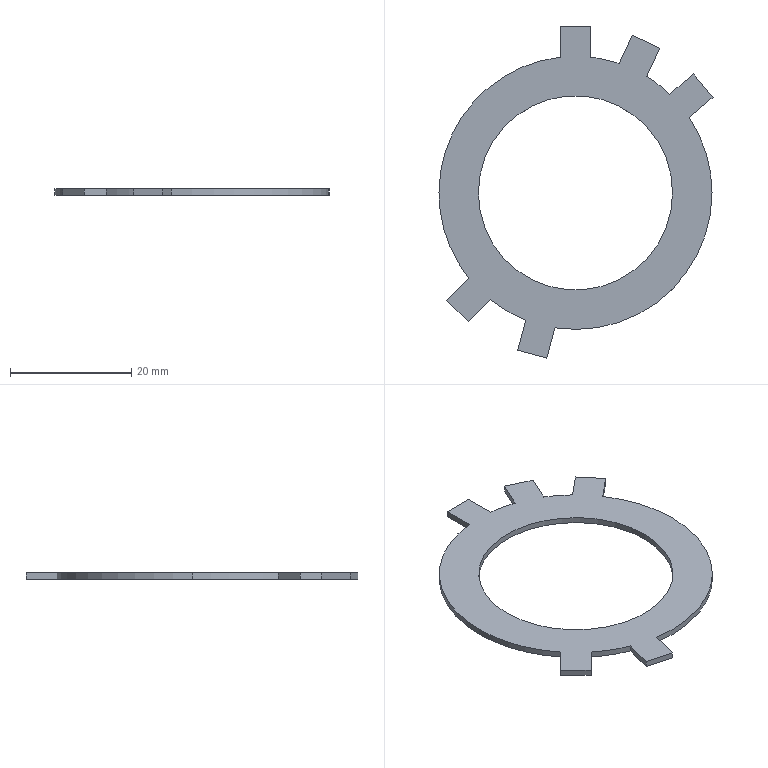Part | STEP file | ZDDQ | 1 solid | 26 faces | box 45.173 x 54.71 x 1 mm | volume 912.343 mm3 | plane 17 | cylinder 9 | commonest cylinder face diameters 45 x7 32 x2
STEP:
#1=CARTESIAN_POINT('',(-9.532,-25.916,0.));
#2=VERTEX_POINT('',#1);
#3=CARTESIAN_POINT('',(-4.703,-27.21,0.));
#4=VERTEX_POINT('',#3);
#5=CARTESIAN_POINT('',(-7.118,-26.563,0.));
#6=DIRECTION('',(-0.9659,0.2588,0.));
#7=VECTOR('',#6,1.);
#8=LINE('',#5,#7);
#9=EDGE_CURVE('',#2,#4,#8,.F.);
#10=ORIENTED_EDGE('',*,*,#9,.T.);
#11=CARTESIAN_POINT('',(-4.703,-27.21,1.));
#12=VERTEX_POINT('',#11);
#13=CARTESIAN_POINT('',(-4.703,-27.21,0.5));
#14=DIRECTION('',(0.,0.,-1.));
#15=VECTOR('',#14,1.);
#16=LINE('',#13,#15);
#17=EDGE_CURVE('',#12,#4,#16,.T.);
#18=ORIENTED_EDGE('',*,*,#17,.F.);
#19=CARTESIAN_POINT('',(-9.532,-25.916,1.));
#20=VERTEX_POINT('',#19);
#21=CARTESIAN_POINT('',(-7.118,-26.563,1.));
#22=DIRECTION('',(-0.9659,0.2588,0.));
#23=VECTOR('',#22,1.);
#24=LINE('',#21,#23);
#25=EDGE_CURVE('',#20,#12,#24,.F.);
#26=ORIENTED_EDGE('',*,*,#25,.F.);
#27=CARTESIAN_POINT('',(-9.532,-25.916,0.5));
#28=DIRECTION('',(0.,0.,-1.));
#29=VECTOR('',#28,1.);
#30=LINE('',#27,#29);
#31=EDGE_CURVE('',#20,#2,#30,.T.);
#32=ORIENTED_EDGE('',*,*,#31,.T.);
#33=EDGE_LOOP('',(#10,#18,#26,#32));
#34=FACE_OUTER_BOUND('',#33,.T.);
#35=CARTESIAN_POINT('',(-4.703,-27.21,1.));
#36=DIRECTION('',(-0.2588,-0.9659,0.));
#37=DIRECTION('',(-0.9659,0.2588,0.));
#38=AXIS2_PLACEMENT_3D('',#35,#36,#37);
#39=PLANE('',#38);
#40=ADVANCED_FACE('',(#34),#39,.T.);
#41=CARTESIAN_POINT('',(-3.373,-22.246,0.));
#42=VERTEX_POINT('',#41);
#43=CARTESIAN_POINT('',(-3.373,-22.246,1.));
#44=VERTEX_POINT('',#43);
#45=CARTESIAN_POINT('',(-3.373,-22.246,0.5));
#46=DIRECTION('',(0.,0.,1.));
#47=VECTOR('',#46,1.);
#48=LINE('',#45,#47);
#49=EDGE_CURVE('',#42,#44,#48,.T.);
#50=ORIENTED_EDGE('',*,*,#49,.T.);
#51=CARTESIAN_POINT('',(-4.038,-24.728,1.));
#52=DIRECTION('',(0.2588,0.9659,0.));
#53=VECTOR('',#52,1.);
#54=LINE('',#51,#53);
#55=EDGE_CURVE('',#12,#44,#54,.T.);
#56=ORIENTED_EDGE('',*,*,#55,.F.);
#57=ORIENTED_EDGE('',*,*,#17,.T.);
#58=CARTESIAN_POINT('',(-4.038,-24.728,0.));
#59=DIRECTION('',(0.2588,0.9659,0.));
#60=VECTOR('',#59,1.);
#61=LINE('',#58,#60);
#62=EDGE_CURVE('',#4,#42,#61,.T.);
#63=ORIENTED_EDGE('',*,*,#62,.T.);
#64=EDGE_LOOP('',(#50,#56,#57,#63));
#65=FACE_OUTER_BOUND('',#64,.T.);
#66=CARTESIAN_POINT('',(-4.703,-27.21,1.));
#67=DIRECTION('',(-0.9659,0.2588,0.));
#68=DIRECTION('',(0.2588,0.9659,0.));
#69=AXIS2_PLACEMENT_3D('',#66,#67,#68);
#70=PLANE('',#69);
#71=ADVANCED_FACE('',(#65),#70,.F.);
#72=CARTESIAN_POINT('',(-8.202,-20.952,0.));
#73=VERTEX_POINT('',#72);
#74=CARTESIAN_POINT('',(-8.202,-20.952,1.));
#75=VERTEX_POINT('',#74);
#76=CARTESIAN_POINT('',(-8.202,-20.952,0.5));
#77=DIRECTION('',(0.,0.,1.));
#78=VECTOR('',#77,1.);
#79=LINE('',#76,#78);
#80=EDGE_CURVE('',#73,#75,#79,.T.);
#81=ORIENTED_EDGE('',*,*,#80,.F.);
#82=CARTESIAN_POINT('',(-8.867,-23.434,0.));
#83=DIRECTION('',(-0.2588,-0.9659,0.));
#84=VECTOR('',#83,1.);
#85=LINE('',#82,#84);
#86=EDGE_CURVE('',#73,#2,#85,.T.);
#87=ORIENTED_EDGE('',*,*,#86,.T.);
#88=ORIENTED_EDGE('',*,*,#31,.F.);
#89=CARTESIAN_POINT('',(-8.867,-23.434,1.));
#90=DIRECTION('',(-0.2588,-0.9659,0.));
#91=VECTOR('',#90,1.);
#92=LINE('',#89,#91);
#93=EDGE_CURVE('',#75,#20,#92,.T.);
#94=ORIENTED_EDGE('',*,*,#93,.F.);
#95=EDGE_LOOP('',(#81,#87,#88,#94));
#96=FACE_OUTER_BOUND('',#95,.T.);
#97=CARTESIAN_POINT('',(-6.944,-16.257,1.));
#98=DIRECTION('',(0.9659,-0.2588,0.));
#99=DIRECTION('',(-0.2588,-0.9659,0.));
#100=AXIS2_PLACEMENT_3D('',#97,#98,#99);
#101=PLANE('',#100);
#102=ADVANCED_FACE('',(#96),#101,.F.);
#103=CARTESIAN_POINT('',(-21.213,-17.678,0.));
#104=VERTEX_POINT('',#103);
#105=CARTESIAN_POINT('',(-17.678,-21.213,0.));
#106=VERTEX_POINT('',#105);
#107=CARTESIAN_POINT('',(-19.445,-19.445,0.));
#108=DIRECTION('',(-0.7071,0.7071,0.));
#109=VECTOR('',#108,1.);
#110=LINE('',#107,#109);
#111=EDGE_CURVE('',#104,#106,#110,.F.);
#112=ORIENTED_EDGE('',*,*,#111,.T.);
#113=CARTESIAN_POINT('',(-17.678,-21.213,1.));
#114=VERTEX_POINT('',#113);
#115=CARTESIAN_POINT('',(-17.678,-21.213,0.5));
#116=DIRECTION('',(0.,0.,-1.));
#117=VECTOR('',#116,1.);
#118=LINE('',#115,#117);
#119=EDGE_CURVE('',#114,#106,#118,.T.);
#120=ORIENTED_EDGE('',*,*,#119,.F.);
#121=CARTESIAN_POINT('',(-21.213,-17.678,1.));
#122=VERTEX_POINT('',#121);
#123=CARTESIAN_POINT('',(-19.445,-19.445,1.));
#124=DIRECTION('',(-0.7071,0.7071,0.));
#125=VECTOR('',#124,1.);
#126=LINE('',#123,#125);
#127=EDGE_CURVE('',#122,#114,#126,.F.);
#128=ORIENTED_EDGE('',*,*,#127,.F.);
#129=CARTESIAN_POINT('',(-21.213,-17.678,0.5));
#130=DIRECTION('',(0.,0.,-1.));
#131=VECTOR('',#130,1.);
#132=LINE('',#129,#131);
#133=EDGE_CURVE('',#122,#104,#132,.T.);
#134=ORIENTED_EDGE('',*,*,#133,.T.);
#135=EDGE_LOOP('',(#112,#120,#128,#134));
#136=FACE_OUTER_BOUND('',#135,.T.);
#137=CARTESIAN_POINT('',(-17.678,-21.213,1.));
#138=DIRECTION('',(-0.7071,-0.7071,0.));
#139=DIRECTION('',(-0.7071,0.7071,0.));
#140=AXIS2_PLACEMENT_3D('',#137,#138,#139);
#141=PLANE('',#140);
#142=ADVANCED_FACE('',(#136),#141,.T.);
#143=CARTESIAN_POINT('',(-14.044,-17.579,0.));
#144=VERTEX_POINT('',#143);
#145=CARTESIAN_POINT('',(-14.044,-17.579,1.));
#146=VERTEX_POINT('',#145);
#147=CARTESIAN_POINT('',(-14.044,-17.579,0.5));
#148=DIRECTION('',(0.,0.,1.));
#149=VECTOR('',#148,1.);
#150=LINE('',#147,#149);
#151=EDGE_CURVE('',#144,#146,#150,.T.);
#152=ORIENTED_EDGE('',*,*,#151,.T.);
#153=CARTESIAN_POINT('',(-15.861,-19.396,1.));
#154=DIRECTION('',(0.7071,0.7071,0.));
#155=VECTOR('',#154,1.);
#156=LINE('',#153,#155);
#157=EDGE_CURVE('',#114,#146,#156,.T.);
#158=ORIENTED_EDGE('',*,*,#157,.F.);
#159=ORIENTED_EDGE('',*,*,#119,.T.);
#160=CARTESIAN_POINT('',(-15.861,-19.396,0.));
#161=DIRECTION('',(0.7071,0.7071,0.));
#162=VECTOR('',#161,1.);
#163=LINE('',#160,#162);
#164=EDGE_CURVE('',#106,#144,#163,.T.);
#165=ORIENTED_EDGE('',*,*,#164,.T.);
#166=EDGE_LOOP('',(#152,#158,#159,#165));
#167=FACE_OUTER_BOUND('',#166,.T.);
#168=CARTESIAN_POINT('',(-17.678,-21.213,1.));
#169=DIRECTION('',(-0.7071,0.7071,0.));
#170=DIRECTION('',(0.7071,0.7071,0.));
#171=AXIS2_PLACEMENT_3D('',#168,#169,#170);
#172=PLANE('',#171);
#173=ADVANCED_FACE('',(#167),#172,.F.);
#174=CARTESIAN_POINT('',(-17.579,-14.044,0.));
#175=VERTEX_POINT('',#174);
#176=CARTESIAN_POINT('',(-17.579,-14.044,1.));
#177=VERTEX_POINT('',#176);
#178=CARTESIAN_POINT('',(-17.579,-14.044,0.5));
#179=DIRECTION('',(0.,0.,1.));
#180=VECTOR('',#179,1.);
#181=LINE('',#178,#180);
#182=EDGE_CURVE('',#175,#177,#181,.T.);
#183=ORIENTED_EDGE('',*,*,#182,.F.);
#184=CARTESIAN_POINT('',(-19.396,-15.861,0.));
#185=DIRECTION('',(-0.7071,-0.7071,0.));
#186=VECTOR('',#185,1.);
#187=LINE('',#184,#186);
#188=EDGE_CURVE('',#175,#104,#187,.T.);
#189=ORIENTED_EDGE('',*,*,#188,.T.);
#190=ORIENTED_EDGE('',*,*,#133,.F.);
#191=CARTESIAN_POINT('',(-19.396,-15.861,1.));
#192=DIRECTION('',(-0.7071,-0.7071,0.));
#193=VECTOR('',#192,1.);
#194=LINE('',#191,#193);
#195=EDGE_CURVE('',#177,#122,#194,.T.);
#196=ORIENTED_EDGE('',*,*,#195,.F.);
#197=EDGE_LOOP('',(#183,#189,#190,#196));
#198=FACE_OUTER_BOUND('',#197,.T.);
#199=CARTESIAN_POINT('',(-14.142,-10.607,1.));
#200=DIRECTION('',(0.7071,-0.7071,0.));
#201=DIRECTION('',(-0.7071,-0.7071,0.));
#202=AXIS2_PLACEMENT_3D('',#199,#200,#201);
#203=PLANE('',#202);
#204=ADVANCED_FACE('',(#198),#203,.F.);
#205=CARTESIAN_POINT('',(13.888,23.867,0.));
#206=VERTEX_POINT('',#205);
#207=CARTESIAN_POINT('',(9.356,25.98,0.));
#208=VERTEX_POINT('',#207);
#209=CARTESIAN_POINT('',(11.622,24.923,0.));
#210=DIRECTION('',(0.9063,-0.4226,0.));
#211=VECTOR('',#210,1.);
#212=LINE('',#209,#211);
#213=EDGE_CURVE('',#206,#208,#212,.F.);
#214=ORIENTED_EDGE('',*,*,#213,.T.);
#215=CARTESIAN_POINT('',(9.356,25.98,1.));
#216=VERTEX_POINT('',#215);
#217=CARTESIAN_POINT('',(9.356,25.98,0.5));
#218=DIRECTION('',(0.,0.,-1.));
#219=VECTOR('',#218,1.);
#220=LINE('',#217,#219);
#221=EDGE_CURVE('',#216,#208,#220,.T.);
#222=ORIENTED_EDGE('',*,*,#221,.F.);
#223=CARTESIAN_POINT('',(13.888,23.867,1.));
#224=VERTEX_POINT('',#223);
#225=CARTESIAN_POINT('',(11.622,24.923,1.));
#226=DIRECTION('',(0.9063,-0.4226,0.));
#227=VECTOR('',#226,1.);
#228=LINE('',#225,#227);
#229=EDGE_CURVE('',#224,#216,#228,.F.);
#230=ORIENTED_EDGE('',*,*,#229,.F.);
#231=CARTESIAN_POINT('',(13.888,23.867,0.5));
#232=DIRECTION('',(0.,0.,-1.));
#233=VECTOR('',#232,1.);
#234=LINE('',#231,#233);
#235=EDGE_CURVE('',#224,#206,#234,.T.);
#236=ORIENTED_EDGE('',*,*,#235,.T.);
#237=EDGE_LOOP('',(#214,#222,#230,#236));
#238=FACE_OUTER_BOUND('',#237,.T.);
#239=CARTESIAN_POINT('',(9.356,25.98,1.));
#240=DIRECTION('',(0.4226,0.9063,0.));
#241=DIRECTION('',(0.9063,-0.4226,0.));
#242=AXIS2_PLACEMENT_3D('',#239,#240,#241);
#243=PLANE('',#242);
#244=ADVANCED_FACE('',(#238),#243,.T.);
#245=CARTESIAN_POINT('',(7.184,21.322,0.));
#246=VERTEX_POINT('',#245);
#247=CARTESIAN_POINT('',(7.184,21.322,1.));
#248=VERTEX_POINT('',#247);
#249=CARTESIAN_POINT('',(7.184,21.322,0.5));
#250=DIRECTION('',(0.,0.,1.));
#251=VECTOR('',#250,1.);
#252=LINE('',#249,#251);
#253=EDGE_CURVE('',#246,#248,#252,.T.);
#254=ORIENTED_EDGE('',*,*,#253,.T.);
#255=CARTESIAN_POINT('',(8.27,23.651,1.));
#256=DIRECTION('',(-0.4226,-0.9063,0.));
#257=VECTOR('',#256,1.);
#258=LINE('',#255,#257);
#259=EDGE_CURVE('',#216,#248,#258,.T.);
#260=ORIENTED_EDGE('',*,*,#259,.F.);
#261=ORIENTED_EDGE('',*,*,#221,.T.);
#262=CARTESIAN_POINT('',(8.27,23.651,0.));
#263=DIRECTION('',(-0.4226,-0.9063,0.));
#264=VECTOR('',#263,1.);
#265=LINE('',#262,#264);
#266=EDGE_CURVE('',#208,#246,#265,.T.);
#267=ORIENTED_EDGE('',*,*,#266,.T.);
#268=EDGE_LOOP('',(#254,#260,#261,#267));
#269=FACE_OUTER_BOUND('',#268,.T.);
#270=CARTESIAN_POINT('',(9.356,25.98,1.));
#271=DIRECTION('',(0.9063,-0.4226,0.));
#272=DIRECTION('',(-0.4226,-0.9063,0.));
#273=AXIS2_PLACEMENT_3D('',#270,#271,#272);
#274=PLANE('',#273);
#275=ADVANCED_FACE('',(#269),#274,.F.);
#276=CARTESIAN_POINT('',(11.716,19.209,0.));
#277=VERTEX_POINT('',#276);
#278=CARTESIAN_POINT('',(11.716,19.209,1.));
#279=VERTEX_POINT('',#278);
#280=CARTESIAN_POINT('',(11.716,19.209,0.5));
#281=DIRECTION('',(0.,0.,1.));
#282=VECTOR('',#281,1.);
#283=LINE('',#280,#282);
#284=EDGE_CURVE('',#277,#279,#283,.T.);
#285=ORIENTED_EDGE('',*,*,#284,.F.);
#286=CARTESIAN_POINT('',(12.802,21.538,0.));
#287=DIRECTION('',(0.4226,0.9063,0.));
#288=VECTOR('',#287,1.);
#289=LINE('',#286,#288);
#290=EDGE_CURVE('',#277,#206,#289,.T.);
#291=ORIENTED_EDGE('',*,*,#290,.T.);
#292=ORIENTED_EDGE('',*,*,#235,.F.);
#293=CARTESIAN_POINT('',(12.802,21.538,1.));
#294=DIRECTION('',(0.4226,0.9063,0.));
#295=VECTOR('',#294,1.);
#296=LINE('',#293,#295);
#297=EDGE_CURVE('',#279,#224,#296,.T.);
#298=ORIENTED_EDGE('',*,*,#297,.F.);
#299=EDGE_LOOP('',(#285,#291,#292,#298));
#300=FACE_OUTER_BOUND('',#299,.T.);
#301=CARTESIAN_POINT('',(9.662,14.804,1.));
#302=DIRECTION('',(-0.9063,0.4226,0.));
#303=DIRECTION('',(0.4226,0.9063,0.));
#304=AXIS2_PLACEMENT_3D('',#301,#302,#303);
#305=PLANE('',#304);
#306=ADVANCED_FACE('',(#300),#305,.F.);
#307=CARTESIAN_POINT('',(22.673,15.762,0.));
#308=VERTEX_POINT('',#307);
#309=CARTESIAN_POINT('',(19.459,19.592,0.));
#310=VERTEX_POINT('',#309);
#311=CARTESIAN_POINT('',(21.066,17.677,0.));
#312=DIRECTION('',(0.6428,-0.766,0.));
#313=VECTOR('',#312,1.);
#314=LINE('',#311,#313);
#315=EDGE_CURVE('',#308,#310,#314,.F.);
#316=ORIENTED_EDGE('',*,*,#315,.T.);
#317=CARTESIAN_POINT('',(19.459,19.592,1.));
#318=VERTEX_POINT('',#317);
#319=CARTESIAN_POINT('',(19.459,19.592,0.5));
#320=DIRECTION('',(0.,0.,-1.));
#321=VECTOR('',#320,1.);
#322=LINE('',#319,#321);
#323=EDGE_CURVE('',#318,#310,#322,.T.);
#324=ORIENTED_EDGE('',*,*,#323,.F.);
#325=CARTESIAN_POINT('',(22.673,15.762,1.));
#326=VERTEX_POINT('',#325);
#327=CARTESIAN_POINT('',(21.066,17.677,1.));
#328=DIRECTION('',(0.6428,-0.766,0.));
#329=VECTOR('',#328,1.);
#330=LINE('',#327,#329);
#331=EDGE_CURVE('',#326,#318,#330,.F.);
#332=ORIENTED_EDGE('',*,*,#331,.F.);
#333=CARTESIAN_POINT('',(22.673,15.762,0.5));
#334=DIRECTION('',(0.,0.,-1.));
#335=VECTOR('',#334,1.);
#336=LINE('',#333,#335);
#337=EDGE_CURVE('',#326,#308,#336,.T.);
#338=ORIENTED_EDGE('',*,*,#337,.T.);
#339=EDGE_LOOP('',(#316,#324,#332,#338));
#340=FACE_OUTER_BOUND('',#339,.T.);
#341=CARTESIAN_POINT('',(19.459,19.592,1.));
#342=DIRECTION('',(0.766,0.6428,0.));
#343=DIRECTION('',(0.6428,-0.766,0.));
#344=AXIS2_PLACEMENT_3D('',#341,#342,#343);
#345=PLANE('',#344);
#346=ADVANCED_FACE('',(#340),#345,.T.);
#347=CARTESIAN_POINT('',(15.522,16.288,0.));
#348=VERTEX_POINT('',#347);
#349=CARTESIAN_POINT('',(15.522,16.288,1.));
#350=VERTEX_POINT('',#349);
#351=CARTESIAN_POINT('',(15.522,16.288,0.5));
#352=DIRECTION('',(0.,0.,1.));
#353=VECTOR('',#352,1.);
#354=LINE('',#351,#353);
#355=EDGE_CURVE('',#348,#350,#354,.T.);
#356=ORIENTED_EDGE('',*,*,#355,.T.);
#357=CARTESIAN_POINT('',(17.491,17.94,1.));
#358=DIRECTION('',(-0.766,-0.6428,0.));
#359=VECTOR('',#358,1.);
#360=LINE('',#357,#359);
#361=EDGE_CURVE('',#318,#350,#360,.T.);
#362=ORIENTED_EDGE('',*,*,#361,.F.);
#363=ORIENTED_EDGE('',*,*,#323,.T.);
#364=CARTESIAN_POINT('',(17.491,17.94,0.));
#365=DIRECTION('',(-0.766,-0.6428,0.));
#366=VECTOR('',#365,1.);
#367=LINE('',#364,#366);
#368=EDGE_CURVE('',#310,#348,#367,.T.);
#369=ORIENTED_EDGE('',*,*,#368,.T.);
#370=EDGE_LOOP('',(#356,#362,#363,#369));
#371=FACE_OUTER_BOUND('',#370,.T.);
#372=CARTESIAN_POINT('',(19.459,19.592,1.));
#373=DIRECTION('',(0.6428,-0.766,0.));
#374=DIRECTION('',(-0.766,-0.6428,0.));
#375=AXIS2_PLACEMENT_3D('',#372,#373,#374);
#376=PLANE('',#375);
#377=ADVANCED_FACE('',(#371),#376,.F.);
#378=CARTESIAN_POINT('',(18.736,12.458,0.));
#379=VERTEX_POINT('',#378);
#380=CARTESIAN_POINT('',(18.736,12.458,1.));
#381=VERTEX_POINT('',#380);
#382=CARTESIAN_POINT('',(18.736,12.458,0.5));
#383=DIRECTION('',(0.,0.,1.));
#384=VECTOR('',#383,1.);
#385=LINE('',#382,#384);
#386=EDGE_CURVE('',#379,#381,#385,.T.);
#387=ORIENTED_EDGE('',*,*,#386,.F.);
#388=CARTESIAN_POINT('',(20.705,14.11,0.));
#389=DIRECTION('',(0.766,0.6428,0.));
#390=VECTOR('',#389,1.);
#391=LINE('',#388,#390);
#392=EDGE_CURVE('',#379,#308,#391,.T.);
#393=ORIENTED_EDGE('',*,*,#392,.T.);
#394=ORIENTED_EDGE('',*,*,#337,.F.);
#395=CARTESIAN_POINT('',(20.705,14.11,1.));
#396=DIRECTION('',(0.766,0.6428,0.));
#397=VECTOR('',#396,1.);
#398=LINE('',#395,#397);
#399=EDGE_CURVE('',#381,#326,#398,.T.);
#400=ORIENTED_EDGE('',*,*,#399,.F.);
#401=EDGE_LOOP('',(#387,#393,#394,#400));
#402=FACE_OUTER_BOUND('',#401,.T.);
#403=CARTESIAN_POINT('',(15.013,9.334,1.));
#404=DIRECTION('',(-0.6428,0.766,0.));
#405=DIRECTION('',(0.766,0.6428,0.));
#406=AXIS2_PLACEMENT_3D('',#403,#404,#405);
#407=PLANE('',#406);
#408=ADVANCED_FACE('',(#402),#407,.F.);
#409=CARTESIAN_POINT('',(-16.,0.,1.));
#410=VERTEX_POINT('',#409);
#411=CARTESIAN_POINT('',(16.,0.,1.));
#412=VERTEX_POINT('',#411);
#413=CARTESIAN_POINT('',(0.,0.,1.));
#414=DIRECTION('',(0.,0.,1.));
#415=AXIS2_PLACEMENT_3D('',#413,#414,$);
#416=CIRCLE('',#415,16.);
#417=EDGE_CURVE('',#410,#412,#416,.T.);
#418=ORIENTED_EDGE('',*,*,#417,.T.);
#419=CARTESIAN_POINT('',(16.,0.,0.));
#420=VERTEX_POINT('',#419);
#421=CARTESIAN_POINT('',(16.,0.,0.5));
#422=DIRECTION('',(0.,0.,1.));
#423=VECTOR('',#422,1.);
#424=LINE('',#421,#423);
#425=EDGE_CURVE('',#420,#412,#424,.T.);
#426=ORIENTED_EDGE('',*,*,#425,.F.);
#427=CARTESIAN_POINT('',(-16.,0.,0.));
#428=VERTEX_POINT('',#427);
#429=CARTESIAN_POINT('',(0.,0.,0.));
#430=DIRECTION('',(0.,0.,1.));
#431=AXIS2_PLACEMENT_3D('',#429,#430,$);
#432=CIRCLE('',#431,16.);
#433=EDGE_CURVE('',#428,#420,#432,.T.);
#434=ORIENTED_EDGE('',*,*,#433,.F.);
#435=CARTESIAN_POINT('',(-16.,0.,0.5));
#436=DIRECTION('',(0.,0.,1.));
#437=VECTOR('',#436,1.);
#438=LINE('',#435,#437);
#439=EDGE_CURVE('',#428,#410,#438,.T.);
#440=ORIENTED_EDGE('',*,*,#439,.T.);
#441=EDGE_LOOP('',(#418,#426,#434,#440));
#442=FACE_OUTER_BOUND('',#441,.T.);
#443=CARTESIAN_POINT('',(0.,0.,0.5));
#444=DIRECTION('',(0.,0.,1.));
#445=DIRECTION('',(1.,0.,0.));
#446=AXIS2_PLACEMENT_3D('',#443,#444,#445);
#447=CYLINDRICAL_SURFACE('',#446,16.);
#448=ADVANCED_FACE('',(#442),#447,.F.);
#449=CARTESIAN_POINT('',(0.,0.,1.));
#450=DIRECTION('',(0.,0.,1.));
#451=AXIS2_PLACEMENT_3D('',#449,#450,$);
#452=CIRCLE('',#451,16.);
#453=EDGE_CURVE('',#412,#410,#452,.T.);
#454=ORIENTED_EDGE('',*,*,#453,.T.);
#455=ORIENTED_EDGE('',*,*,#439,.F.);
#456=CARTESIAN_POINT('',(0.,0.,0.));
#457=DIRECTION('',(0.,0.,1.));
#458=AXIS2_PLACEMENT_3D('',#456,#457,$);
#459=CIRCLE('',#458,16.);
#460=EDGE_CURVE('',#420,#428,#459,.T.);
#461=ORIENTED_EDGE('',*,*,#460,.F.);
#462=ORIENTED_EDGE('',*,*,#425,.T.);
#463=EDGE_LOOP('',(#454,#455,#461,#462));
#464=FACE_OUTER_BOUND('',#463,.T.);
#465=ADVANCED_FACE('',(#464),#447,.F.);
#466=CARTESIAN_POINT('',(0.,0.,0.));
#467=DIRECTION('',(0.,0.,1.));
#468=AXIS2_PLACEMENT_3D('',#466,#467,$);
#469=CIRCLE('',#468,22.5);
#470=EDGE_CURVE('',#348,#277,#469,.T.);
#471=ORIENTED_EDGE('',*,*,#470,.T.);
#472=ORIENTED_EDGE('',*,*,#284,.T.);
#473=CARTESIAN_POINT('',(0.,0.,1.));
#474=DIRECTION('',(0.,0.,1.));
#475=AXIS2_PLACEMENT_3D('',#473,#474,$);
#476=CIRCLE('',#475,22.5);
#477=EDGE_CURVE('',#350,#279,#476,.T.);
#478=ORIENTED_EDGE('',*,*,#477,.F.);
#479=ORIENTED_EDGE('',*,*,#355,.F.);
#480=EDGE_LOOP('',(#471,#472,#478,#479));
#481=FACE_OUTER_BOUND('',#480,.T.);
#482=CARTESIAN_POINT('',(0.,0.,0.5));
#483=DIRECTION('',(0.,0.,1.));
#484=DIRECTION('',(1.,0.,0.));
#485=AXIS2_PLACEMENT_3D('',#482,#483,#484);
#486=CYLINDRICAL_SURFACE('',#485,22.5);
#487=ADVANCED_FACE('',(#481),#486,.T.);
#488=ORIENTED_EDGE('',*,*,#253,.F.);
#489=CARTESIAN_POINT('',(2.5,22.361,0.));
#490=VERTEX_POINT('',#489);
#491=CARTESIAN_POINT('',(0.,0.,0.));
#492=DIRECTION('',(0.,0.,1.));
#493=AXIS2_PLACEMENT_3D('',#491,#492,$);
#494=CIRCLE('',#493,22.5);
#495=EDGE_CURVE('',#246,#490,#494,.T.);
#496=ORIENTED_EDGE('',*,*,#495,.T.);
#497=CARTESIAN_POINT('',(2.5,22.361,1.));
#498=VERTEX_POINT('',#497);
#499=CARTESIAN_POINT('',(2.5,22.361,0.5));
#500=DIRECTION('',(0.,0.,1.));
#501=VECTOR('',#500,1.);
#502=LINE('',#499,#501);
#503=EDGE_CURVE('',#490,#498,#502,.T.);
#504=ORIENTED_EDGE('',*,*,#503,.T.);
#505=CARTESIAN_POINT('',(0.,0.,1.));
#506=DIRECTION('',(0.,0.,1.));
#507=AXIS2_PLACEMENT_3D('',#505,#506,$);
#508=CIRCLE('',#507,22.5);
#509=EDGE_CURVE('',#248,#498,#508,.T.);
#510=ORIENTED_EDGE('',*,*,#509,.F.);
#511=EDGE_LOOP('',(#488,#496,#504,#510));
#512=FACE_OUTER_BOUND('',#511,.T.);
#513=ADVANCED_FACE('',(#512),#486,.T.);
#514=CARTESIAN_POINT('',(-2.5,22.361,0.));
#515=VERTEX_POINT('',#514);
#516=CARTESIAN_POINT('',(-22.5,0.,0.));
#517=VERTEX_POINT('',#516);
#518=CARTESIAN_POINT('',(0.,0.,0.));
#519=DIRECTION('',(0.,0.,1.));
#520=AXIS2_PLACEMENT_3D('',#518,#519,$);
#521=CIRCLE('',#520,22.5);
#522=EDGE_CURVE('',#515,#517,#521,.T.);
#523=ORIENTED_EDGE('',*,*,#522,.T.);
#524=CARTESIAN_POINT('',(-22.5,0.,1.));
#525=VERTEX_POINT('',#524);
#526=CARTESIAN_POINT('',(-22.5,0.,0.5));
#527=DIRECTION('',(0.,0.,1.));
#528=VECTOR('',#527,1.);
#529=LINE('',#526,#528);
#530=EDGE_CURVE('',#517,#525,#529,.T.);
#531=ORIENTED_EDGE('',*,*,#530,.T.);
#532=CARTESIAN_POINT('',(-2.5,22.361,1.));
#533=VERTEX_POINT('',#532);
#534=CARTESIAN_POINT('',(0.,0.,1.));
#535=DIRECTION('',(0.,0.,1.));
#536=AXIS2_PLACEMENT_3D('',#534,#535,$);
#537=CIRCLE('',#536,22.5);
#538=EDGE_CURVE('',#533,#525,#537,.T.);
#539=ORIENTED_EDGE('',*,*,#538,.F.);
#540=CARTESIAN_POINT('',(-2.5,22.361,0.5));
#541=DIRECTION('',(0.,0.,1.));
#542=VECTOR('',#541,1.);
#543=LINE('',#540,#542);
#544=EDGE_CURVE('',#515,#533,#543,.T.);
#545=ORIENTED_EDGE('',*,*,#544,.F.);
#546=EDGE_LOOP('',(#523,#531,#539,#545));
#547=FACE_OUTER_BOUND('',#546,.T.);
#548=ADVANCED_FACE('',(#547),#486,.T.);
#549=CARTESIAN_POINT('',(0.,0.,1.));
#550=DIRECTION('',(0.,0.,1.));
#551=AXIS2_PLACEMENT_3D('',#549,#550,$);
#552=CIRCLE('',#551,22.5);
#553=EDGE_CURVE('',#525,#177,#552,.T.);
#554=ORIENTED_EDGE('',*,*,#553,.F.);
#555=ORIENTED_EDGE('',*,*,#530,.F.);
#556=CARTESIAN_POINT('',(0.,0.,0.));
#557=DIRECTION('',(0.,0.,1.));
#558=AXIS2_PLACEMENT_3D('',#556,#557,$);
#559=CIRCLE('',#558,22.5);
#560=EDGE_CURVE('',#517,#175,#559,.T.);
#561=ORIENTED_EDGE('',*,*,#560,.T.);
#562=ORIENTED_EDGE('',*,*,#182,.T.);
#563=EDGE_LOOP('',(#554,#555,#561,#562));
#564=FACE_OUTER_BOUND('',#563,.T.);
#565=ADVANCED_FACE('',(#564),#486,.T.);
#566=CARTESIAN_POINT('',(0.,0.,0.));
#567=DIRECTION('',(0.,0.,1.));
#568=AXIS2_PLACEMENT_3D('',#566,#567,$);
#569=CIRCLE('',#568,22.5);
#570=EDGE_CURVE('',#144,#73,#569,.T.);
#571=ORIENTED_EDGE('',*,*,#570,.T.);
#572=ORIENTED_EDGE('',*,*,#80,.T.);
#573=CARTESIAN_POINT('',(0.,0.,1.));
#574=DIRECTION('',(0.,0.,1.));
#575=AXIS2_PLACEMENT_3D('',#573,#574,$);
#576=CIRCLE('',#575,22.5);
#577=EDGE_CURVE('',#146,#75,#576,.T.);
#578=ORIENTED_EDGE('',*,*,#577,.F.);
#579=ORIENTED_EDGE('',*,*,#151,.F.);
#580=EDGE_LOOP('',(#571,#572,#578,#579));
#581=FACE_OUTER_BOUND('',#580,.T.);
#582=ADVANCED_FACE('',(#581),#486,.T.);
#583=CARTESIAN_POINT('',(22.5,0.,0.));
#584=VERTEX_POINT('',#583);
#585=CARTESIAN_POINT('',(0.,0.,0.));
#586=DIRECTION('',(0.,0.,1.));
#587=AXIS2_PLACEMENT_3D('',#585,#586,$);
#588=CIRCLE('',#587,22.5);
#589=EDGE_CURVE('',#42,#584,#588,.T.);
#590=ORIENTED_EDGE('',*,*,#589,.T.);
#591=CARTESIAN_POINT('',(22.5,0.,1.));
#592=VERTEX_POINT('',#591);
#593=CARTESIAN_POINT('',(22.5,0.,0.5));
#594=DIRECTION('',(0.,0.,1.));
#595=VECTOR('',#594,1.);
#596=LINE('',#593,#595);
#597=EDGE_CURVE('',#584,#592,#596,.T.);
#598=ORIENTED_EDGE('',*,*,#597,.T.);
#599=CARTESIAN_POINT('',(0.,0.,1.));
#600=DIRECTION('',(0.,0.,1.));
#601=AXIS2_PLACEMENT_3D('',#599,#600,$);
#602=CIRCLE('',#601,22.5);
#603=EDGE_CURVE('',#44,#592,#602,.T.);
#604=ORIENTED_EDGE('',*,*,#603,.F.);
#605=ORIENTED_EDGE('',*,*,#49,.F.);
#606=EDGE_LOOP('',(#590,#598,#604,#605));
#607=FACE_OUTER_BOUND('',#606,.T.);
#608=ADVANCED_FACE('',(#607),#486,.T.);
#609=CARTESIAN_POINT('',(0.,0.,1.));
#610=DIRECTION('',(0.,0.,1.));
#611=AXIS2_PLACEMENT_3D('',#609,#610,$);
#612=CIRCLE('',#611,22.5);
#613=EDGE_CURVE('',#592,#381,#612,.T.);
#614=ORIENTED_EDGE('',*,*,#613,.F.);
#615=ORIENTED_EDGE('',*,*,#597,.F.);
#616=CARTESIAN_POINT('',(0.,0.,0.));
#617=DIRECTION('',(0.,0.,1.));
#618=AXIS2_PLACEMENT_3D('',#616,#617,$);
#619=CIRCLE('',#618,22.5);
#620=EDGE_CURVE('',#584,#379,#619,.T.);
#621=ORIENTED_EDGE('',*,*,#620,.T.);
#622=ORIENTED_EDGE('',*,*,#386,.T.);
#623=EDGE_LOOP('',(#614,#615,#621,#622));
#624=FACE_OUTER_BOUND('',#623,.T.);
#625=ADVANCED_FACE('',(#624),#486,.T.);
#626=CARTESIAN_POINT('',(2.5,27.5,0.));
#627=VERTEX_POINT('',#626);
#628=CARTESIAN_POINT('',(-2.5,27.5,0.));
#629=VERTEX_POINT('',#628);
#630=CARTESIAN_POINT('',(0.,27.5,0.));
#631=DIRECTION('',(1.,0.,0.));
#632=VECTOR('',#631,1.);
#633=LINE('',#630,#632);
#634=EDGE_CURVE('',#627,#629,#633,.F.);
#635=ORIENTED_EDGE('',*,*,#634,.T.);
#636=CARTESIAN_POINT('',(-2.5,27.5,1.));
#637=VERTEX_POINT('',#636);
#638=CARTESIAN_POINT('',(-2.5,27.5,0.5));
#639=DIRECTION('',(0.,0.,-1.));
#640=VECTOR('',#639,1.);
#641=LINE('',#638,#640);
#642=EDGE_CURVE('',#637,#629,#641,.T.);
#643=ORIENTED_EDGE('',*,*,#642,.F.);
#644=CARTESIAN_POINT('',(2.5,27.5,1.));
#645=VERTEX_POINT('',#644);
#646=CARTESIAN_POINT('',(0.,27.5,1.));
#647=DIRECTION('',(1.,0.,0.));
#648=VECTOR('',#647,1.);
#649=LINE('',#646,#648);
#650=EDGE_CURVE('',#645,#637,#649,.F.);
#651=ORIENTED_EDGE('',*,*,#650,.F.);
#652=CARTESIAN_POINT('',(2.5,27.5,0.5));
#653=DIRECTION('',(0.,0.,-1.));
#654=VECTOR('',#653,1.);
#655=LINE('',#652,#654);
#656=EDGE_CURVE('',#645,#627,#655,.T.);
#657=ORIENTED_EDGE('',*,*,#656,.T.);
#658=EDGE_LOOP('',(#635,#643,#651,#657));
#659=FACE_OUTER_BOUND('',#658,.T.);
#660=CARTESIAN_POINT('',(-2.5,27.5,1.));
#661=DIRECTION('',(0.,1.,0.));
#662=DIRECTION('',(1.,0.,0.));
#663=AXIS2_PLACEMENT_3D('',#660,#661,#662);
#664=PLANE('',#663);
#665=ADVANCED_FACE('',(#659),#664,.T.);
#666=ORIENTED_EDGE('',*,*,#544,.T.);
#667=CARTESIAN_POINT('',(-2.5,24.93,1.));
#668=DIRECTION('',(0.,-1.,0.));
#669=VECTOR('',#668,1.);
#670=LINE('',#667,#669);
#671=EDGE_CURVE('',#637,#533,#670,.T.);
#672=ORIENTED_EDGE('',*,*,#671,.F.);
#673=ORIENTED_EDGE('',*,*,#642,.T.);
#674=CARTESIAN_POINT('',(-2.5,24.93,0.));
#675=DIRECTION('',(0.,-1.,0.));
#676=VECTOR('',#675,1.);
#677=LINE('',#674,#676);
#678=EDGE_CURVE('',#629,#515,#677,.T.);
#679=ORIENTED_EDGE('',*,*,#678,.T.);
#680=EDGE_LOOP('',(#666,#672,#673,#679));
#681=FACE_OUTER_BOUND('',#680,.T.);
#682=CARTESIAN_POINT('',(-2.5,27.5,1.));
#683=DIRECTION('',(1.,0.,0.));
#684=DIRECTION('',(0.,-1.,0.));
#685=AXIS2_PLACEMENT_3D('',#682,#683,#684);
#686=PLANE('',#685);
#687=ADVANCED_FACE('',(#681),#686,.F.);
#688=ORIENTED_EDGE('',*,*,#503,.F.);
#689=CARTESIAN_POINT('',(2.5,24.93,0.));
#690=DIRECTION('',(0.,1.,0.));
#691=VECTOR('',#690,1.);
#692=LINE('',#689,#691);
#693=EDGE_CURVE('',#490,#627,#692,.T.);
#694=ORIENTED_EDGE('',*,*,#693,.T.);
#695=ORIENTED_EDGE('',*,*,#656,.F.);
#696=CARTESIAN_POINT('',(2.5,24.93,1.));
#697=DIRECTION('',(0.,1.,0.));
#698=VECTOR('',#697,1.);
#699=LINE('',#696,#698);
#700=EDGE_CURVE('',#498,#645,#699,.T.);
#701=ORIENTED_EDGE('',*,*,#700,.F.);
#702=EDGE_LOOP('',(#688,#694,#695,#701));
#703=FACE_OUTER_BOUND('',#702,.T.);
#704=CARTESIAN_POINT('',(2.5,17.5,1.));
#705=DIRECTION('',(-1.,0.,0.));
#706=DIRECTION('',(0.,1.,0.));
#707=AXIS2_PLACEMENT_3D('',#704,#705,#706);
#708=PLANE('',#707);
#709=ADVANCED_FACE('',(#703),#708,.F.);
#710=ORIENTED_EDGE('',*,*,#495,.F.);
#711=ORIENTED_EDGE('',*,*,#266,.F.);
#712=ORIENTED_EDGE('',*,*,#213,.F.);
#713=ORIENTED_EDGE('',*,*,#290,.F.);
#714=ORIENTED_EDGE('',*,*,#470,.F.);
#715=ORIENTED_EDGE('',*,*,#368,.F.);
#716=ORIENTED_EDGE('',*,*,#315,.F.);
#717=ORIENTED_EDGE('',*,*,#392,.F.);
#718=ORIENTED_EDGE('',*,*,#620,.F.);
#719=ORIENTED_EDGE('',*,*,#589,.F.);
#720=ORIENTED_EDGE('',*,*,#62,.F.);
#721=ORIENTED_EDGE('',*,*,#9,.F.);
#722=ORIENTED_EDGE('',*,*,#86,.F.);
#723=ORIENTED_EDGE('',*,*,#570,.F.);
#724=ORIENTED_EDGE('',*,*,#164,.F.);
#725=ORIENTED_EDGE('',*,*,#111,.F.);
#726=ORIENTED_EDGE('',*,*,#188,.F.);
#727=ORIENTED_EDGE('',*,*,#560,.F.);
#728=ORIENTED_EDGE('',*,*,#522,.F.);
#729=ORIENTED_EDGE('',*,*,#678,.F.);
#730=ORIENTED_EDGE('',*,*,#634,.F.);
#731=ORIENTED_EDGE('',*,*,#693,.F.);
#732=EDGE_LOOP('',(#710,#711,#712,#713,#714,#715,#716,#717,#718,#719,#720,#721,#722,#723,#724,#725,#726,#727,#728,#729,#730,#731));
#733=FACE_OUTER_BOUND('',#732,.T.);
#734=ORIENTED_EDGE('',*,*,#433,.T.);
#735=ORIENTED_EDGE('',*,*,#460,.T.);
#736=EDGE_LOOP('',(#734,#735));
#737=FACE_BOUND('',#736,.T.);
#738=CARTESIAN_POINT('',(0.,0.,0.));
#739=DIRECTION('',(0.,0.,1.));
#740=DIRECTION('',(1.,0.,0.));
#741=AXIS2_PLACEMENT_3D('',#738,#739,#740);
#742=PLANE('',#741);
#743=ADVANCED_FACE('',(#733,#737),#742,.F.);
#744=ORIENTED_EDGE('',*,*,#700,.T.);
#745=ORIENTED_EDGE('',*,*,#650,.T.);
#746=ORIENTED_EDGE('',*,*,#671,.T.);
#747=ORIENTED_EDGE('',*,*,#538,.T.);
#748=ORIENTED_EDGE('',*,*,#553,.T.);
#749=ORIENTED_EDGE('',*,*,#195,.T.);
#750=ORIENTED_EDGE('',*,*,#127,.T.);
#751=ORIENTED_EDGE('',*,*,#157,.T.);
#752=ORIENTED_EDGE('',*,*,#577,.T.);
#753=ORIENTED_EDGE('',*,*,#93,.T.);
#754=ORIENTED_EDGE('',*,*,#25,.T.);
#755=ORIENTED_EDGE('',*,*,#55,.T.);
#756=ORIENTED_EDGE('',*,*,#603,.T.);
#757=ORIENTED_EDGE('',*,*,#613,.T.);
#758=ORIENTED_EDGE('',*,*,#399,.T.);
#759=ORIENTED_EDGE('',*,*,#331,.T.);
#760=ORIENTED_EDGE('',*,*,#361,.T.);
#761=ORIENTED_EDGE('',*,*,#477,.T.);
#762=ORIENTED_EDGE('',*,*,#297,.T.);
#763=ORIENTED_EDGE('',*,*,#229,.T.);
#764=ORIENTED_EDGE('',*,*,#259,.T.);
#765=ORIENTED_EDGE('',*,*,#509,.T.);
#766=EDGE_LOOP('',(#744,#745,#746,#747,#748,#749,#750,#751,#752,#753,#754,#755,#756,#757,#758,#759,#760,#761,#762,#763,#764,#765));
#767=FACE_OUTER_BOUND('',#766,.T.);
#768=ORIENTED_EDGE('',*,*,#453,.F.);
#769=ORIENTED_EDGE('',*,*,#417,.F.);
#770=EDGE_LOOP('',(#768,#769));
#771=FACE_BOUND('',#770,.T.);
#772=CARTESIAN_POINT('',(0.,0.,1.));
#773=DIRECTION('',(0.,0.,1.));
#774=DIRECTION('',(1.,0.,0.));
#775=AXIS2_PLACEMENT_3D('',#772,#773,#774);
#776=PLANE('',#775);
#777=ADVANCED_FACE('',(#767,#771),#776,.T.);
#778=CLOSED_SHELL('',(#40,#71,#102,#142,#173,#204,#244,#275,#306,#346,#377,#408,#448,#465,#487,#513,#548,#565,#582,#608,#625,#665,#687,#709,#743,#777));
#779=MANIFOLD_SOLID_BREP('',#778);
#780=(LENGTH_UNIT()NAMED_UNIT(*)SI_UNIT(.MILLI.,.METRE.));
#781=UNCERTAINTY_MEASURE_WITH_UNIT(LENGTH_MEASURE(0.005),#780,'','');
#782=(NAMED_UNIT(*)PLANE_ANGLE_UNIT()SI_UNIT($,.RADIAN.));
#783=(NAMED_UNIT(*)SI_UNIT($,.STERADIAN.)SOLID_ANGLE_UNIT());
#784=(GEOMETRIC_REPRESENTATION_CONTEXT(3)GLOBAL_UNCERTAINTY_ASSIGNED_CONTEXT((#781))GLOBAL_UNIT_ASSIGNED_CONTEXT((#780,#782,#783))REPRESENTATION_CONTEXT('',''));
#785=ADVANCED_BREP_SHAPE_REPRESENTATION('',(#779),#784);